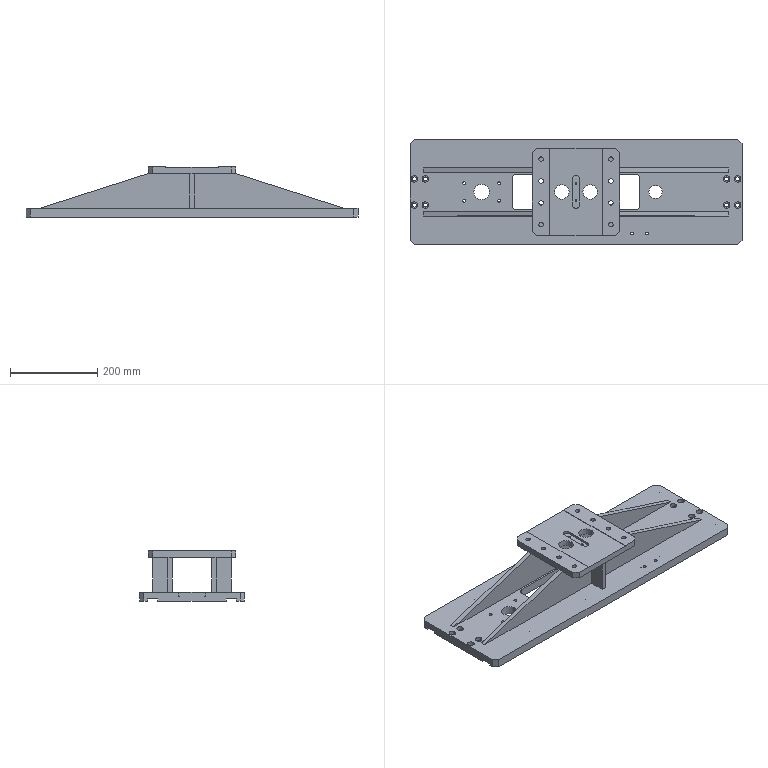Part | STEP file | YCD14007A-08.03.02 Clamping Slide | 1 solid | 247 faces | box 760 x 240 x 115 mm | volume 4249230 mm3 | cylinder 130 | plane 65 | cone 52 | commonest cylinder face diameters 5 x52 9 x16 10.2 x16 15 x16 6.8 x12 4.2 x4